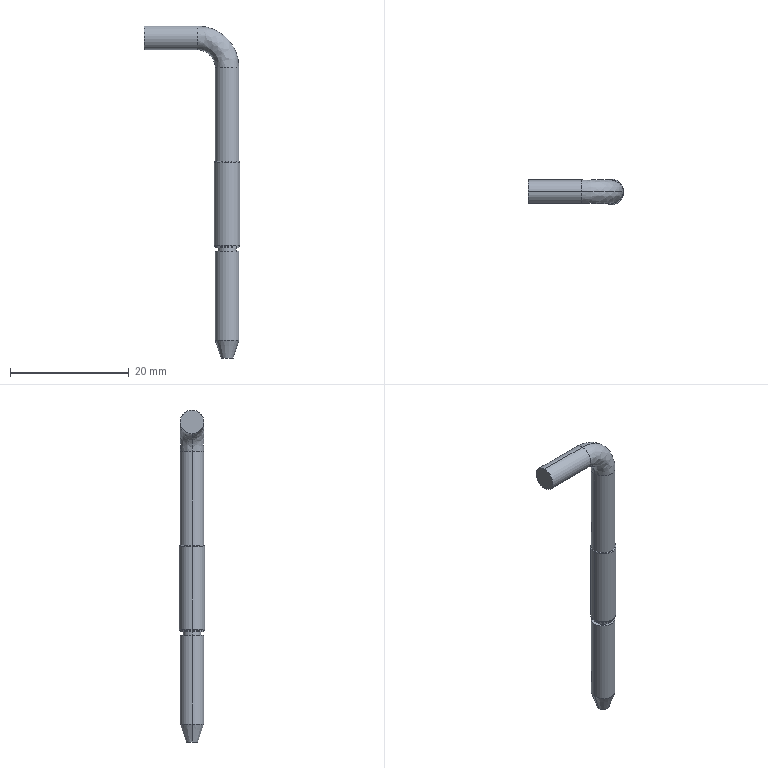Part | SolidWorks | features MirrorStock 1 | 1 solid | 24 faces | box 16.15 x 4.3 x 56 mm | volume 836.376 mm3 | cylinder 12 | spline 6 | plane 4 | cone 2 | commonest cylinder face diameters 4 x8 3 x2 4.3 x2
STEP:
#1=CARTESIAN_POINT('',(-2.,4.,7.15));
#2=VERTEX_POINT('',#1);
#3=CARTESIAN_POINT('',(2.,4.,7.15));
#4=VERTEX_POINT('',#3);
#5=CARTESIAN_POINT('',(0.,4.,7.15));
#6=DIRECTION('',(0.,0.,-1.));
#7=DIRECTION('',(-1.,0.,0.));
#8=AXIS2_PLACEMENT_3D('',#5,#6,#7);
#9=CIRCLE('',#8,2.);
#10=EDGE_CURVE('',#2,#4,#9,.T.);
#11=ORIENTED_EDGE('',*,*,#10,.T.);
#12=CARTESIAN_POINT('',(2.15,4.,7.));
#13=VERTEX_POINT('',#12);
#14=CARTESIAN_POINT('',(2.,4.,7.));
#15=DIRECTION('',(0.,1.,0.));
#16=DIRECTION('',(1.,0.,0.));
#17=AXIS2_PLACEMENT_3D('',#14,#15,#16);
#18=CIRCLE('',#17,0.15);
#19=EDGE_CURVE('',#4,#13,#18,.T.);
#20=ORIENTED_EDGE('',*,*,#19,.T.);
#21=CARTESIAN_POINT('',(-2.15,4.,7.));
#22=VERTEX_POINT('',#21);
#23=CARTESIAN_POINT('',(0.,4.,7.));
#24=DIRECTION('',(0.,0.,-1.));
#25=DIRECTION('',(-1.,0.,0.));
#26=AXIS2_PLACEMENT_3D('',#23,#24,#25);
#27=CIRCLE('',#26,2.15);
#28=EDGE_CURVE('',#22,#13,#27,.T.);
#29=ORIENTED_EDGE('',*,*,#28,.F.);
#30=CARTESIAN_POINT('',(-2.,4.,7.));
#31=DIRECTION('',(0.,-1.,0.));
#32=DIRECTION('',(-1.,0.,0.));
#33=AXIS2_PLACEMENT_3D('',#30,#31,#32);
#34=CIRCLE('',#33,0.15);
#35=EDGE_CURVE('',#2,#22,#34,.T.);
#36=ORIENTED_EDGE('',*,*,#35,.F.);
#37=EDGE_LOOP('',(#11,#20,#29,#36));
#38=FACE_OUTER_BOUND('',#37,.T.);
#39=CARTESIAN_POINT('',(2.,4.,7.15));
#40=CARTESIAN_POINT('',(2.,8.,7.15));
#41=CARTESIAN_POINT('',(-2.,8.,7.15));
#42=CARTESIAN_POINT('',(-2.,4.,7.15));
#43=CARTESIAN_POINT('',(2.088,4.,7.15));
#44=CARTESIAN_POINT('',(2.088,8.176,7.15));
#45=CARTESIAN_POINT('',(-2.088,8.176,7.15));
#46=CARTESIAN_POINT('',(-2.088,4.,7.15));
#47=CARTESIAN_POINT('',(2.15,4.,7.088));
#48=CARTESIAN_POINT('',(2.15,8.3,7.088));
#49=CARTESIAN_POINT('',(-2.15,8.3,7.088));
#50=CARTESIAN_POINT('',(-2.15,4.,7.088));
#51=CARTESIAN_POINT('',(2.15,4.,7.));
#52=CARTESIAN_POINT('',(2.15,8.3,7.));
#53=CARTESIAN_POINT('',(-2.15,8.3,7.));
#54=CARTESIAN_POINT('',(-2.15,4.,7.));
#55=(BOUNDED_SURFACE()B_SPLINE_SURFACE(3,3,((#39,#40,#41,#42),(#43,#44,#45,#46),(#47,#48,#49,#50),(#51,#52,#53,#54)),.UNSPECIFIED.,.F.,.F.,.T.)B_SPLINE_SURFACE_WITH_KNOTS((4,4),(4,4),(0.,1.),(0.,1.),.UNSPECIFIED.)GEOMETRIC_REPRESENTATION_ITEM()RATIONAL_B_SPLINE_SURFACE(((1.,0.3333,0.3333,1.),(0.8047,0.2682,0.2682,0.8047),(0.8047,0.2682,0.2682,0.8047),(1.,0.3333,0.3333,1.)))REPRESENTATION_ITEM('')SURFACE());
#56=ADVANCED_FACE('',(#38),#55,.T.);
#57=CARTESIAN_POINT('',(-2.15,4.,-7.));
#58=VERTEX_POINT('',#57);
#59=CARTESIAN_POINT('',(2.15,4.,-7.));
#60=VERTEX_POINT('',#59);
#61=CARTESIAN_POINT('',(0.,4.,-7.));
#62=DIRECTION('',(0.,0.,-1.));
#63=DIRECTION('',(-1.,0.,0.));
#64=AXIS2_PLACEMENT_3D('',#61,#62,#63);
#65=CIRCLE('',#64,2.15);
#66=EDGE_CURVE('',#58,#60,#65,.T.);
#67=ORIENTED_EDGE('',*,*,#66,.T.);
#68=CARTESIAN_POINT('',(2.,4.,-7.15));
#69=VERTEX_POINT('',#68);
#70=CARTESIAN_POINT('',(2.,4.,-7.));
#71=DIRECTION('',(0.,1.,0.));
#72=DIRECTION('',(1.,0.,0.));
#73=AXIS2_PLACEMENT_3D('',#70,#71,#72);
#74=CIRCLE('',#73,0.15);
#75=EDGE_CURVE('',#60,#69,#74,.T.);
#76=ORIENTED_EDGE('',*,*,#75,.T.);
#77=CARTESIAN_POINT('',(-2.,4.,-7.15));
#78=VERTEX_POINT('',#77);
#79=CARTESIAN_POINT('',(0.,4.,-7.15));
#80=DIRECTION('',(0.,0.,-1.));
#81=DIRECTION('',(-1.,0.,0.));
#82=AXIS2_PLACEMENT_3D('',#79,#80,#81);
#83=CIRCLE('',#82,2.);
#84=EDGE_CURVE('',#78,#69,#83,.T.);
#85=ORIENTED_EDGE('',*,*,#84,.F.);
#86=CARTESIAN_POINT('',(-2.,4.,-7.));
#87=DIRECTION('',(0.,-1.,0.));
#88=DIRECTION('',(-1.,0.,0.));
#89=AXIS2_PLACEMENT_3D('',#86,#87,#88);
#90=CIRCLE('',#89,0.15);
#91=EDGE_CURVE('',#58,#78,#90,.T.);
#92=ORIENTED_EDGE('',*,*,#91,.F.);
#93=EDGE_LOOP('',(#67,#76,#85,#92));
#94=FACE_OUTER_BOUND('',#93,.T.);
#95=CARTESIAN_POINT('',(2.15,4.,-7.));
#96=CARTESIAN_POINT('',(2.15,8.3,-7.));
#97=CARTESIAN_POINT('',(-2.15,8.3,-7.));
#98=CARTESIAN_POINT('',(-2.15,4.,-7.));
#99=CARTESIAN_POINT('',(2.15,4.,-7.088));
#100=CARTESIAN_POINT('',(2.15,8.3,-7.088));
#101=CARTESIAN_POINT('',(-2.15,8.3,-7.088));
#102=CARTESIAN_POINT('',(-2.15,4.,-7.088));
#103=CARTESIAN_POINT('',(2.088,4.,-7.15));
#104=CARTESIAN_POINT('',(2.088,8.176,-7.15));
#105=CARTESIAN_POINT('',(-2.088,8.176,-7.15));
#106=CARTESIAN_POINT('',(-2.088,4.,-7.15));
#107=CARTESIAN_POINT('',(2.,4.,-7.15));
#108=CARTESIAN_POINT('',(2.,8.,-7.15));
#109=CARTESIAN_POINT('',(-2.,8.,-7.15));
#110=CARTESIAN_POINT('',(-2.,4.,-7.15));
#111=(BOUNDED_SURFACE()B_SPLINE_SURFACE(3,3,((#95,#96,#97,#98),(#99,#100,#101,#102),(#103,#104,#105,#106),(#107,#108,#109,#110)),.UNSPECIFIED.,.F.,.F.,.T.)B_SPLINE_SURFACE_WITH_KNOTS((4,4),(4,4),(0.,1.),(0.,1.),.UNSPECIFIED.)GEOMETRIC_REPRESENTATION_ITEM()RATIONAL_B_SPLINE_SURFACE(((1.,0.3333,0.3333,1.),(0.8047,0.2682,0.2682,0.8047),(0.8047,0.2682,0.2682,0.8047),(1.,0.3333,0.3333,1.)))REPRESENTATION_ITEM('')SURFACE());
#112=ADVANCED_FACE('',(#94),#111,.T.);
#113=CARTESIAN_POINT('',(0.,4.,7.15));
#114=DIRECTION('',(0.,0.,-1.));
#115=DIRECTION('',(-1.,0.,0.));
#116=AXIS2_PLACEMENT_3D('',#113,#114,#115);
#117=CIRCLE('',#116,2.);
#118=EDGE_CURVE('',#4,#2,#117,.T.);
#119=ORIENTED_EDGE('',*,*,#118,.F.);
#120=CARTESIAN_POINT('',(2.,4.,23.));
#121=VERTEX_POINT('',#120);
#122=CARTESIAN_POINT('',(2.,4.,23.));
#123=DIRECTION('',(0.,0.,1.));
#124=VECTOR('',#123,1000.);
#125=LINE('',#122,#124);
#126=EDGE_CURVE('',#4,#121,#125,.T.);
#127=ORIENTED_EDGE('',*,*,#126,.T.);
#128=CARTESIAN_POINT('',(-2.,4.,23.));
#129=VERTEX_POINT('',#128);
#130=CARTESIAN_POINT('',(0.,4.,23.));
#131=DIRECTION('',(0.,0.,1.));
#132=DIRECTION('',(-1.,0.,0.));
#133=AXIS2_PLACEMENT_3D('',#130,#131,#132);
#134=CIRCLE('',#133,2.);
#135=EDGE_CURVE('',#129,#121,#134,.T.);
#136=ORIENTED_EDGE('',*,*,#135,.F.);
#137=CARTESIAN_POINT('',(-2.,4.,23.));
#138=DIRECTION('',(0.,0.,1.));
#139=VECTOR('',#138,1000.);
#140=LINE('',#137,#139);
#141=EDGE_CURVE('',#2,#129,#140,.T.);
#142=ORIENTED_EDGE('',*,*,#141,.F.);
#143=EDGE_LOOP('',(#119,#127,#136,#142));
#144=FACE_OUTER_BOUND('',#143,.T.);
#145=CARTESIAN_POINT('',(0.,4.,23.));
#146=DIRECTION('',(0.,0.,1.));
#147=DIRECTION('',(-1.,0.,0.));
#148=AXIS2_PLACEMENT_3D('',#145,#146,#147);
#149=CYLINDRICAL_SURFACE('',#148,2.);
#150=ADVANCED_FACE('',(#144),#149,.T.);
#151=CARTESIAN_POINT('',(-5.,4.,26.));
#152=VERTEX_POINT('',#151);
#153=CARTESIAN_POINT('',(-5.,4.,30.));
#154=VERTEX_POINT('',#153);
#155=CARTESIAN_POINT('',(-5.,4.,28.));
#156=DIRECTION('',(-1.,0.,0.));
#157=DIRECTION('',(0.,0.,1.));
#158=AXIS2_PLACEMENT_3D('',#155,#156,#157);
#159=CIRCLE('',#158,2.);
#160=EDGE_CURVE('',#152,#154,#159,.T.);
#161=ORIENTED_EDGE('',*,*,#160,.F.);
#162=CARTESIAN_POINT('',(-5.,4.,23.));
#163=DIRECTION('',(0.,1.,0.));
#164=DIRECTION('',(0.,0.,-1.));
#165=AXIS2_PLACEMENT_3D('',#162,#163,#164);
#166=CIRCLE('',#165,3.);
#167=EDGE_CURVE('',#152,#129,#166,.T.);
#168=ORIENTED_EDGE('',*,*,#167,.T.);
#169=ORIENTED_EDGE('',*,*,#135,.T.);
#170=CARTESIAN_POINT('',(-5.,4.,23.));
#171=DIRECTION('',(0.,1.,0.));
#172=DIRECTION('',(0.,0.,-1.));
#173=AXIS2_PLACEMENT_3D('',#170,#171,#172);
#174=CIRCLE('',#173,7.);
#175=EDGE_CURVE('',#154,#121,#174,.T.);
#176=ORIENTED_EDGE('',*,*,#175,.F.);
#177=EDGE_LOOP('',(#161,#168,#169,#176));
#178=FACE_OUTER_BOUND('',#177,.T.);
#179=CARTESIAN_POINT('',(-5.,4.,30.));
#180=CARTESIAN_POINT('',(-0.8995,4.,30.));
#181=CARTESIAN_POINT('',(2.,4.,27.101));
#182=CARTESIAN_POINT('',(2.,4.,23.));
#183=CARTESIAN_POINT('',(-5.,0.,30.));
#184=CARTESIAN_POINT('',(-0.8995,0.,30.));
#185=CARTESIAN_POINT('',(2.,0.,27.101));
#186=CARTESIAN_POINT('',(2.,0.,23.));
#187=CARTESIAN_POINT('',(-5.,0.,26.));
#188=CARTESIAN_POINT('',(-3.243,0.,26.));
#189=CARTESIAN_POINT('',(-2.,0.,24.757));
#190=CARTESIAN_POINT('',(-2.,0.,23.));
#191=CARTESIAN_POINT('',(-5.,4.,26.));
#192=CARTESIAN_POINT('',(-3.243,4.,26.));
#193=CARTESIAN_POINT('',(-2.,4.,24.757));
#194=CARTESIAN_POINT('',(-2.,4.,23.));
#195=(BOUNDED_SURFACE()B_SPLINE_SURFACE(3,3,((#179,#180,#181,#182),(#183,#184,#185,#186),(#187,#188,#189,#190),(#191,#192,#193,#194)),.UNSPECIFIED.,.F.,.F.,.T.)B_SPLINE_SURFACE_WITH_KNOTS((4,4),(4,4),(0.,1.),(0.,1.),.UNSPECIFIED.)GEOMETRIC_REPRESENTATION_ITEM()RATIONAL_B_SPLINE_SURFACE(((1.,0.8047,0.8047,1.),(0.3333,0.2682,0.2682,0.3333),(0.3333,0.2682,0.2682,0.3333),(1.,0.8047,0.8047,1.)))REPRESENTATION_ITEM('')SURFACE());
#196=ADVANCED_FACE('',(#178),#195,.T.);
#197=CARTESIAN_POINT('',(0.,4.,-7.));
#198=DIRECTION('',(0.,0.,-1.));
#199=DIRECTION('',(-1.,0.,0.));
#200=AXIS2_PLACEMENT_3D('',#197,#198,#199);
#201=CIRCLE('',#200,2.15);
#202=EDGE_CURVE('',#60,#58,#201,.T.);
#203=ORIENTED_EDGE('',*,*,#202,.F.);
#204=CARTESIAN_POINT('',(2.15,4.,-7.));
#205=DIRECTION('',(0.,0.,1.));
#206=VECTOR('',#205,1000.);
#207=LINE('',#204,#206);
#208=EDGE_CURVE('',#60,#13,#207,.T.);
#209=ORIENTED_EDGE('',*,*,#208,.T.);
#210=CARTESIAN_POINT('',(0.,4.,7.));
#211=DIRECTION('',(0.,0.,-1.));
#212=DIRECTION('',(-1.,0.,0.));
#213=AXIS2_PLACEMENT_3D('',#210,#211,#212);
#214=CIRCLE('',#213,2.15);
#215=EDGE_CURVE('',#13,#22,#214,.T.);
#216=ORIENTED_EDGE('',*,*,#215,.T.);
#217=CARTESIAN_POINT('',(-2.15,4.,-7.));
#218=DIRECTION('',(0.,0.,1.));
#219=VECTOR('',#218,1000.);
#220=LINE('',#217,#219);
#221=EDGE_CURVE('',#58,#22,#220,.T.);
#222=ORIENTED_EDGE('',*,*,#221,.F.);
#223=EDGE_LOOP('',(#203,#209,#216,#222));
#224=FACE_OUTER_BOUND('',#223,.T.);
#225=CARTESIAN_POINT('',(0.,4.,-7.));
#226=DIRECTION('',(0.,0.,1.));
#227=DIRECTION('',(-1.,0.,0.));
#228=AXIS2_PLACEMENT_3D('',#225,#226,#227);
#229=CYLINDRICAL_SURFACE('',#228,2.15);
#230=ADVANCED_FACE('',(#224),#229,.T.);
#231=CARTESIAN_POINT('',(-14.,4.,26.));
#232=VERTEX_POINT('',#231);
#233=CARTESIAN_POINT('',(-14.,4.,30.));
#234=VERTEX_POINT('',#233);
#235=CARTESIAN_POINT('',(-14.,4.,28.));
#236=DIRECTION('',(-1.,0.,0.));
#237=DIRECTION('',(0.,0.,1.));
#238=AXIS2_PLACEMENT_3D('',#235,#236,#237);
#239=CIRCLE('',#238,2.);
#240=EDGE_CURVE('',#232,#234,#239,.T.);
#241=ORIENTED_EDGE('',*,*,#240,.F.);
#242=CARTESIAN_POINT('',(-14.,4.,26.));
#243=DIRECTION('',(1.,0.,0.));
#244=VECTOR('',#243,1000.);
#245=LINE('',#242,#244);
#246=EDGE_CURVE('',#232,#152,#245,.T.);
#247=ORIENTED_EDGE('',*,*,#246,.T.);
#248=ORIENTED_EDGE('',*,*,#160,.T.);
#249=CARTESIAN_POINT('',(-14.,4.,30.));
#250=DIRECTION('',(1.,0.,0.));
#251=VECTOR('',#250,1000.);
#252=LINE('',#249,#251);
#253=EDGE_CURVE('',#234,#154,#252,.T.);
#254=ORIENTED_EDGE('',*,*,#253,.F.);
#255=EDGE_LOOP('',(#241,#247,#248,#254));
#256=FACE_OUTER_BOUND('',#255,.T.);
#257=CARTESIAN_POINT('',(-14.,4.,28.));
#258=DIRECTION('',(1.,0.,0.));
#259=DIRECTION('',(0.,0.,1.));
#260=AXIS2_PLACEMENT_3D('',#257,#258,#259);
#261=CYLINDRICAL_SURFACE('',#260,2.);
#262=ADVANCED_FACE('',(#256),#261,.T.);
#263=CARTESIAN_POINT('',(2.,4.,-7.4));
#264=VERTEX_POINT('',#263);
#265=CARTESIAN_POINT('',(-2.,4.,-7.4));
#266=VERTEX_POINT('',#265);
#267=CARTESIAN_POINT('',(0.,4.,-7.4));
#268=DIRECTION('',(0.,0.,-1.));
#269=DIRECTION('',(-1.,0.,0.));
#270=AXIS2_PLACEMENT_3D('',#267,#268,#269);
#271=CIRCLE('',#270,2.);
#272=EDGE_CURVE('',#264,#266,#271,.T.);
#273=ORIENTED_EDGE('',*,*,#272,.F.);
#274=CARTESIAN_POINT('',(2.,4.,23.));
#275=DIRECTION('',(0.,0.,1.));
#276=VECTOR('',#275,1000.);
#277=LINE('',#274,#276);
#278=EDGE_CURVE('',#264,#69,#277,.T.);
#279=ORIENTED_EDGE('',*,*,#278,.T.);
#280=CARTESIAN_POINT('',(0.,4.,-7.15));
#281=DIRECTION('',(0.,0.,-1.));
#282=DIRECTION('',(-1.,0.,0.));
#283=AXIS2_PLACEMENT_3D('',#280,#281,#282);
#284=CIRCLE('',#283,2.);
#285=EDGE_CURVE('',#69,#78,#284,.T.);
#286=ORIENTED_EDGE('',*,*,#285,.T.);
#287=CARTESIAN_POINT('',(-2.,4.,23.));
#288=DIRECTION('',(0.,0.,1.));
#289=VECTOR('',#288,1000.);
#290=LINE('',#287,#289);
#291=EDGE_CURVE('',#266,#78,#290,.T.);
#292=ORIENTED_EDGE('',*,*,#291,.F.);
#293=EDGE_LOOP('',(#273,#279,#286,#292));
#294=FACE_OUTER_BOUND('',#293,.T.);
#295=CARTESIAN_POINT('',(0.,4.,23.));
#296=DIRECTION('',(0.,0.,1.));
#297=DIRECTION('',(-1.,0.,0.));
#298=AXIS2_PLACEMENT_3D('',#295,#296,#297);
#299=CYLINDRICAL_SURFACE('',#298,2.);
#300=ADVANCED_FACE('',(#294),#299,.T.);
#301=CARTESIAN_POINT('',(-1.5,4.,-7.4));
#302=VERTEX_POINT('',#301);
#303=CARTESIAN_POINT('',(1.5,4.,-7.4));
#304=VERTEX_POINT('',#303);
#305=CARTESIAN_POINT('',(0.,4.,-7.4));
#306=DIRECTION('',(0.,0.,1.));
#307=DIRECTION('',(1.,0.,0.));
#308=AXIS2_PLACEMENT_3D('',#305,#306,#307);
#309=CIRCLE('',#308,1.5);
#310=EDGE_CURVE('',#302,#304,#309,.T.);
#311=ORIENTED_EDGE('',*,*,#310,.F.);
#312=CARTESIAN_POINT('',(-1.5,4.,-8.));
#313=VERTEX_POINT('',#312);
#314=CARTESIAN_POINT('',(-1.5,4.,-50.));
#315=DIRECTION('',(0.,0.,-1.));
#316=VECTOR('',#315,1000.);
#317=LINE('',#314,#316);
#318=EDGE_CURVE('',#302,#313,#317,.T.);
#319=ORIENTED_EDGE('',*,*,#318,.T.);
#320=CARTESIAN_POINT('',(1.5,4.,-8.));
#321=VERTEX_POINT('',#320);
#322=CARTESIAN_POINT('',(0.,4.,-8.));
#323=DIRECTION('',(0.,0.,-1.));
#324=DIRECTION('',(1.,0.,0.));
#325=AXIS2_PLACEMENT_3D('',#322,#323,#324);
#326=CIRCLE('',#325,1.5);
#327=EDGE_CURVE('',#321,#313,#326,.T.);
#328=ORIENTED_EDGE('',*,*,#327,.F.);
#329=CARTESIAN_POINT('',(1.5,4.,-50.));
#330=DIRECTION('',(0.,0.,-1.));
#331=VECTOR('',#330,1000.);
#332=LINE('',#329,#331);
#333=EDGE_CURVE('',#304,#321,#332,.T.);
#334=ORIENTED_EDGE('',*,*,#333,.F.);
#335=EDGE_LOOP('',(#311,#319,#328,#334));
#336=FACE_OUTER_BOUND('',#335,.T.);
#337=CARTESIAN_POINT('',(0.,4.,-50.));
#338=DIRECTION('',(0.,0.,-1.));
#339=DIRECTION('',(1.,0.,0.));
#340=AXIS2_PLACEMENT_3D('',#337,#338,#339);
#341=CYLINDRICAL_SURFACE('',#340,1.5);
#342=ADVANCED_FACE('',(#336),#341,.T.);
#343=CARTESIAN_POINT('',(2.,4.,-23.));
#344=VERTEX_POINT('',#343);
#345=CARTESIAN_POINT('',(-2.,4.,-23.));
#346=VERTEX_POINT('',#345);
#347=CARTESIAN_POINT('',(0.,4.,-23.));
#348=DIRECTION('',(0.,0.,-1.));
#349=DIRECTION('',(-1.,0.,0.));
#350=AXIS2_PLACEMENT_3D('',#347,#348,#349);
#351=CIRCLE('',#350,2.);
#352=EDGE_CURVE('',#344,#346,#351,.T.);
#353=ORIENTED_EDGE('',*,*,#352,.F.);
#354=CARTESIAN_POINT('',(2.,4.,-8.));
#355=VERTEX_POINT('',#354);
#356=CARTESIAN_POINT('',(2.,4.,23.));
#357=DIRECTION('',(0.,0.,1.));
#358=VECTOR('',#357,1000.);
#359=LINE('',#356,#358);
#360=EDGE_CURVE('',#344,#355,#359,.T.);
#361=ORIENTED_EDGE('',*,*,#360,.T.);
#362=CARTESIAN_POINT('',(-2.,4.,-8.));
#363=VERTEX_POINT('',#362);
#364=CARTESIAN_POINT('',(0.,4.,-8.));
#365=DIRECTION('',(0.,0.,1.));
#366=DIRECTION('',(-1.,0.,0.));
#367=AXIS2_PLACEMENT_3D('',#364,#365,#366);
#368=CIRCLE('',#367,2.);
#369=EDGE_CURVE('',#363,#355,#368,.T.);
#370=ORIENTED_EDGE('',*,*,#369,.F.);
#371=CARTESIAN_POINT('',(-2.,4.,23.));
#372=DIRECTION('',(0.,0.,1.));
#373=VECTOR('',#372,1000.);
#374=LINE('',#371,#373);
#375=EDGE_CURVE('',#346,#363,#374,.T.);
#376=ORIENTED_EDGE('',*,*,#375,.F.);
#377=EDGE_LOOP('',(#353,#361,#370,#376));
#378=FACE_OUTER_BOUND('',#377,.T.);
#379=CARTESIAN_POINT('',(0.,4.,23.));
#380=DIRECTION('',(0.,0.,1.));
#381=DIRECTION('',(-1.,0.,0.));
#382=AXIS2_PLACEMENT_3D('',#379,#380,#381);
#383=CYLINDRICAL_SURFACE('',#382,2.);
#384=ADVANCED_FACE('',(#378),#383,.T.);
#385=CARTESIAN_POINT('',(1.,4.,-26.));
#386=VERTEX_POINT('',#385);
#387=CARTESIAN_POINT('',(-1.,4.,-26.));
#388=VERTEX_POINT('',#387);
#389=CARTESIAN_POINT('',(0.,4.,-26.));
#390=DIRECTION('',(0.,0.,-1.));
#391=DIRECTION('',(-1.,0.,0.));
#392=AXIS2_PLACEMENT_3D('',#389,#390,#391);
#393=CIRCLE('',#392,1.);
#394=EDGE_CURVE('',#386,#388,#393,.T.);
#395=ORIENTED_EDGE('',*,*,#394,.F.);
#396=CARTESIAN_POINT('',(2.,4.,-23.));
#397=DIRECTION('',(0.3162,0.,0.9487));
#398=VECTOR('',#397,1000.);
#399=LINE('',#396,#398);
#400=EDGE_CURVE('',#386,#344,#399,.T.);
#401=ORIENTED_EDGE('',*,*,#400,.T.);
#402=ORIENTED_EDGE('',*,*,#352,.T.);
#403=CARTESIAN_POINT('',(-2.,4.,-23.));
#404=DIRECTION('',(-0.3162,0.,0.9487));
#405=VECTOR('',#404,1000.);
#406=LINE('',#403,#405);
#407=EDGE_CURVE('',#388,#346,#406,.T.);
#408=ORIENTED_EDGE('',*,*,#407,.F.);
#409=EDGE_LOOP('',(#395,#401,#402,#408));
#410=FACE_OUTER_BOUND('',#409,.T.);
#411=CARTESIAN_POINT('',(0.,4.,-23.));
#412=DIRECTION('',(0.,0.,1.));
#413=DIRECTION('',(-1.,0.,0.));
#414=AXIS2_PLACEMENT_3D('',#411,#412,#413);
#415=CONICAL_SURFACE('',#414,2.,0.3218);
#416=ADVANCED_FACE('',(#410),#415,.T.);
#417=CARTESIAN_POINT('',(0.,4.,-26.));
#418=DIRECTION('',(0.,0.,-1.));
#419=DIRECTION('',(-1.,0.,0.));
#420=AXIS2_PLACEMENT_3D('',#417,#418,#419);
#421=CIRCLE('',#420,1.);
#422=EDGE_CURVE('',#388,#386,#421,.T.);
#423=ORIENTED_EDGE('',*,*,#422,.T.);
#424=ORIENTED_EDGE('',*,*,#394,.T.);
#425=EDGE_LOOP('',(#423,#424));
#426=FACE_OUTER_BOUND('',#425,.T.);
#427=CARTESIAN_POINT('',(0.,4.,-26.));
#428=DIRECTION('',(0.,0.,1.));
#429=DIRECTION('',(-1.,0.,0.));
#430=AXIS2_PLACEMENT_3D('',#427,#428,#429);
#431=PLANE('',#430);
#432=ADVANCED_FACE('',(#426),#431,.F.);
#433=ORIENTED_EDGE('',*,*,#400,.F.);
#434=ORIENTED_EDGE('',*,*,#422,.F.);
#435=ORIENTED_EDGE('',*,*,#407,.T.);
#436=CARTESIAN_POINT('',(0.,4.,-23.));
#437=DIRECTION('',(0.,0.,-1.));
#438=DIRECTION('',(-1.,0.,0.));
#439=AXIS2_PLACEMENT_3D('',#436,#437,#438);
#440=CIRCLE('',#439,2.);
#441=EDGE_CURVE('',#346,#344,#440,.T.);
#442=ORIENTED_EDGE('',*,*,#441,.T.);
#443=EDGE_LOOP('',(#433,#434,#435,#442));
#444=FACE_OUTER_BOUND('',#443,.T.);
#445=CARTESIAN_POINT('',(0.,4.,-23.));
#446=DIRECTION('',(0.,0.,1.));
#447=DIRECTION('',(-1.,0.,0.));
#448=AXIS2_PLACEMENT_3D('',#445,#446,#447);
#449=CONICAL_SURFACE('',#448,2.,0.3218);
#450=ADVANCED_FACE('',(#444),#449,.T.);
#451=ORIENTED_EDGE('',*,*,#360,.F.);
#452=ORIENTED_EDGE('',*,*,#441,.F.);
#453=ORIENTED_EDGE('',*,*,#375,.T.);
#454=CARTESIAN_POINT('',(0.,4.,-8.));
#455=DIRECTION('',(0.,0.,1.));
#456=DIRECTION('',(-1.,0.,0.));
#457=AXIS2_PLACEMENT_3D('',#454,#455,#456);
#458=CIRCLE('',#457,2.);
#459=EDGE_CURVE('',#355,#363,#458,.T.);
#460=ORIENTED_EDGE('',*,*,#459,.F.);
#461=EDGE_LOOP('',(#451,#452,#453,#460));
#462=FACE_OUTER_BOUND('',#461,.T.);
#463=CARTESIAN_POINT('',(0.,4.,23.));
#464=DIRECTION('',(0.,0.,1.));
#465=DIRECTION('',(-1.,0.,0.));
#466=AXIS2_PLACEMENT_3D('',#463,#464,#465);
#467=CYLINDRICAL_SURFACE('',#466,2.);
#468=ADVANCED_FACE('',(#462),#467,.T.);
#469=ORIENTED_EDGE('',*,*,#327,.T.);
#470=CARTESIAN_POINT('',(0.,4.,-8.));
#471=DIRECTION('',(0.,0.,-1.));
#472=DIRECTION('',(1.,0.,0.));
#473=AXIS2_PLACEMENT_3D('',#470,#471,#472);
#474=CIRCLE('',#473,1.5);
#475=EDGE_CURVE('',#313,#321,#474,.T.);
#476=ORIENTED_EDGE('',*,*,#475,.T.);
#477=EDGE_LOOP('',(#469,#476));
#478=FACE_BOUND('',#477,.T.);
#479=ORIENTED_EDGE('',*,*,#369,.T.);
#480=ORIENTED_EDGE('',*,*,#459,.T.);
#481=EDGE_LOOP('',(#479,#480));
#482=FACE_OUTER_BOUND('',#481,.T.);
#483=CARTESIAN_POINT('',(1.5,4.,-8.));
#484=DIRECTION('',(0.,0.,-1.));
#485=DIRECTION('',(1.,0.,0.));
#486=AXIS2_PLACEMENT_3D('',#483,#484,#485);
#487=PLANE('',#486);
#488=ADVANCED_FACE('',(#478,#482),#487,.F.);
#489=ORIENTED_EDGE('',*,*,#318,.F.);
#490=CARTESIAN_POINT('',(0.,4.,-7.4));
#491=DIRECTION('',(0.,0.,1.));
#492=DIRECTION('',(1.,0.,0.));
#493=AXIS2_PLACEMENT_3D('',#490,#491,#492);
#494=CIRCLE('',#493,1.5);
#495=EDGE_CURVE('',#304,#302,#494,.T.);
#496=ORIENTED_EDGE('',*,*,#495,.F.);
#497=ORIENTED_EDGE('',*,*,#333,.T.);
#498=ORIENTED_EDGE('',*,*,#475,.F.);
#499=EDGE_LOOP('',(#489,#496,#497,#498));
#500=FACE_OUTER_BOUND('',#499,.T.);
#501=CARTESIAN_POINT('',(0.,4.,-50.));
#502=DIRECTION('',(0.,0.,-1.));
#503=DIRECTION('',(1.,0.,0.));
#504=AXIS2_PLACEMENT_3D('',#501,#502,#503);
#505=CYLINDRICAL_SURFACE('',#504,1.5);
#506=ADVANCED_FACE('',(#500),#505,.T.);
#507=CARTESIAN_POINT('',(0.,4.,-7.4));
#508=DIRECTION('',(0.,0.,-1.));
#509=DIRECTION('',(-1.,0.,0.));
#510=AXIS2_PLACEMENT_3D('',#507,#508,#509);
#511=CIRCLE('',#510,2.);
#512=EDGE_CURVE('',#266,#264,#511,.T.);
#513=ORIENTED_EDGE('',*,*,#512,.T.);
#514=ORIENTED_EDGE('',*,*,#272,.T.);
#515=EDGE_LOOP('',(#513,#514));
#516=FACE_OUTER_BOUND('',#515,.T.);
#517=ORIENTED_EDGE('',*,*,#495,.T.);
#518=ORIENTED_EDGE('',*,*,#310,.T.);
#519=EDGE_LOOP('',(#517,#518));
#520=FACE_BOUND('',#519,.T.);
#521=CARTESIAN_POINT('',(4.,4.,-7.4));
#522=DIRECTION('',(0.,0.,1.));
#523=DIRECTION('',(-1.,0.,0.));
#524=AXIS2_PLACEMENT_3D('',#521,#522,#523);
#525=PLANE('',#524);
#526=ADVANCED_FACE('',(#516,#520),#525,.F.);
#527=ORIENTED_EDGE('',*,*,#278,.F.);
#528=ORIENTED_EDGE('',*,*,#512,.F.);
#529=ORIENTED_EDGE('',*,*,#291,.T.);
#530=ORIENTED_EDGE('',*,*,#84,.T.);
#531=EDGE_LOOP('',(#527,#528,#529,#530));
#532=FACE_OUTER_BOUND('',#531,.T.);
#533=CARTESIAN_POINT('',(0.,4.,23.));
#534=DIRECTION('',(0.,0.,1.));
#535=DIRECTION('',(-1.,0.,0.));
#536=AXIS2_PLACEMENT_3D('',#533,#534,#535);
#537=CYLINDRICAL_SURFACE('',#536,2.);
#538=ADVANCED_FACE('',(#532),#537,.T.);
#539=CARTESIAN_POINT('',(-14.,4.,28.));
#540=DIRECTION('',(-1.,0.,0.));
#541=DIRECTION('',(0.,0.,1.));
#542=AXIS2_PLACEMENT_3D('',#539,#540,#541);
#543=CIRCLE('',#542,2.);
#544=EDGE_CURVE('',#234,#232,#543,.T.);
#545=ORIENTED_EDGE('',*,*,#544,.T.);
#546=ORIENTED_EDGE('',*,*,#240,.T.);
#547=EDGE_LOOP('',(#545,#546));
#548=FACE_OUTER_BOUND('',#547,.T.);
#549=CARTESIAN_POINT('',(-14.,4.,28.));
#550=DIRECTION('',(-1.,0.,0.));
#551=DIRECTION('',(0.,0.,-1.));
#552=AXIS2_PLACEMENT_3D('',#549,#550,#551);
#553=PLANE('',#552);
#554=ADVANCED_FACE('',(#548),#553,.T.);
#555=ORIENTED_EDGE('',*,*,#75,.F.);
#556=ORIENTED_EDGE('',*,*,#202,.T.);
#557=ORIENTED_EDGE('',*,*,#91,.T.);
#558=ORIENTED_EDGE('',*,*,#285,.F.);
#559=EDGE_LOOP('',(#555,#556,#557,#558));
#560=FACE_OUTER_BOUND('',#559,.T.);
#561=CARTESIAN_POINT('',(-2.15,4.,-7.));
#562=CARTESIAN_POINT('',(-2.15,-0.3,-7.));
#563=CARTESIAN_POINT('',(2.15,-0.3,-7.));
#564=CARTESIAN_POINT('',(2.15,4.,-7.));
#565=CARTESIAN_POINT('',(-2.15,4.,-7.088));
#566=CARTESIAN_POINT('',(-2.15,-0.3,-7.088));
#567=CARTESIAN_POINT('',(2.15,-0.3,-7.088));
#568=CARTESIAN_POINT('',(2.15,4.,-7.088));
#569=CARTESIAN_POINT('',(-2.088,4.,-7.15));
#570=CARTESIAN_POINT('',(-2.088,-0.1757,-7.15));
#571=CARTESIAN_POINT('',(2.088,-0.1757,-7.15));
#572=CARTESIAN_POINT('',(2.088,4.,-7.15));
#573=CARTESIAN_POINT('',(-2.,4.,-7.15));
#574=CARTESIAN_POINT('',(-2.,0.,-7.15));
#575=CARTESIAN_POINT('',(2.,0.,-7.15));
#576=CARTESIAN_POINT('',(2.,4.,-7.15));
#577=(BOUNDED_SURFACE()B_SPLINE_SURFACE(3,3,((#561,#562,#563,#564),(#565,#566,#567,#568),(#569,#570,#571,#572),(#573,#574,#575,#576)),.UNSPECIFIED.,.F.,.F.,.T.)B_SPLINE_SURFACE_WITH_KNOTS((4,4),(4,4),(0.,1.),(0.,1.),.UNSPECIFIED.)GEOMETRIC_REPRESENTATION_ITEM()RATIONAL_B_SPLINE_SURFACE(((1.,0.3333,0.3333,1.),(0.8047,0.2682,0.2682,0.8047),(0.8047,0.2682,0.2682,0.8047),(1.,0.3333,0.3333,1.)))REPRESENTATION_ITEM('')SURFACE());
#578=ADVANCED_FACE('',(#560),#577,.T.);
#579=ORIENTED_EDGE('',*,*,#246,.F.);
#580=ORIENTED_EDGE('',*,*,#544,.F.);
#581=ORIENTED_EDGE('',*,*,#253,.T.);
#582=CARTESIAN_POINT('',(-5.,4.,28.));
#583=DIRECTION('',(-1.,0.,0.));
#584=DIRECTION('',(0.,0.,1.));
#585=AXIS2_PLACEMENT_3D('',#582,#583,#584);
#586=CIRCLE('',#585,2.);
#587=EDGE_CURVE('',#154,#152,#586,.T.);
#588=ORIENTED_EDGE('',*,*,#587,.T.);
#589=EDGE_LOOP('',(#579,#580,#581,#588));
#590=FACE_OUTER_BOUND('',#589,.T.);
#591=CARTESIAN_POINT('',(-14.,4.,28.));
#592=DIRECTION('',(1.,0.,0.));
#593=DIRECTION('',(0.,0.,1.));
#594=AXIS2_PLACEMENT_3D('',#591,#592,#593);
#595=CYLINDRICAL_SURFACE('',#594,2.);
#596=ADVANCED_FACE('',(#590),#595,.T.);
#597=ORIENTED_EDGE('',*,*,#208,.F.);
#598=ORIENTED_EDGE('',*,*,#66,.F.);
#599=ORIENTED_EDGE('',*,*,#221,.T.);
#600=ORIENTED_EDGE('',*,*,#28,.T.);
#601=EDGE_LOOP('',(#597,#598,#599,#600));
#602=FACE_OUTER_BOUND('',#601,.T.);
#603=CARTESIAN_POINT('',(0.,4.,-7.));
#604=DIRECTION('',(0.,0.,1.));
#605=DIRECTION('',(-1.,0.,0.));
#606=AXIS2_PLACEMENT_3D('',#603,#604,#605);
#607=CYLINDRICAL_SURFACE('',#606,2.15);
#608=ADVANCED_FACE('',(#602),#607,.T.);
#609=ORIENTED_EDGE('',*,*,#167,.F.);
#610=ORIENTED_EDGE('',*,*,#587,.F.);
#611=ORIENTED_EDGE('',*,*,#175,.T.);
#612=CARTESIAN_POINT('',(0.,4.,23.));
#613=DIRECTION('',(0.,0.,1.));
#614=DIRECTION('',(-1.,0.,0.));
#615=AXIS2_PLACEMENT_3D('',#612,#613,#614);
#616=CIRCLE('',#615,2.);
#617=EDGE_CURVE('',#121,#129,#616,.T.);
#618=ORIENTED_EDGE('',*,*,#617,.T.);
#619=EDGE_LOOP('',(#609,#610,#611,#618));
#620=FACE_OUTER_BOUND('',#619,.T.);
#621=CARTESIAN_POINT('',(-5.,4.,26.));
#622=CARTESIAN_POINT('',(-3.243,4.,26.));
#623=CARTESIAN_POINT('',(-2.,4.,24.757));
#624=CARTESIAN_POINT('',(-2.,4.,23.));
#625=CARTESIAN_POINT('',(-5.,8.,26.));
#626=CARTESIAN_POINT('',(-3.243,8.,26.));
#627=CARTESIAN_POINT('',(-2.,8.,24.757));
#628=CARTESIAN_POINT('',(-2.,8.,23.));
#629=CARTESIAN_POINT('',(-5.,8.,30.));
#630=CARTESIAN_POINT('',(-0.8995,8.,30.));
#631=CARTESIAN_POINT('',(2.,8.,27.101));
#632=CARTESIAN_POINT('',(2.,8.,23.));
#633=CARTESIAN_POINT('',(-5.,4.,30.));
#634=CARTESIAN_POINT('',(-0.8995,4.,30.));
#635=CARTESIAN_POINT('',(2.,4.,27.101));
#636=CARTESIAN_POINT('',(2.,4.,23.));
#637=(BOUNDED_SURFACE()B_SPLINE_SURFACE(3,3,((#621,#622,#623,#624),(#625,#626,#627,#628),(#629,#630,#631,#632),(#633,#634,#635,#636)),.UNSPECIFIED.,.F.,.F.,.T.)B_SPLINE_SURFACE_WITH_KNOTS((4,4),(4,4),(0.,1.),(0.,1.),.UNSPECIFIED.)GEOMETRIC_REPRESENTATION_ITEM()RATIONAL_B_SPLINE_SURFACE(((1.,0.8047,0.8047,1.),(0.3333,0.2682,0.2682,0.3333),(0.3333,0.2682,0.2682,0.3333),(1.,0.8047,0.8047,1.)))REPRESENTATION_ITEM('')SURFACE());
#638=ADVANCED_FACE('',(#620),#637,.T.);
#639=ORIENTED_EDGE('',*,*,#19,.F.);
#640=ORIENTED_EDGE('',*,*,#118,.T.);
#641=ORIENTED_EDGE('',*,*,#35,.T.);
#642=ORIENTED_EDGE('',*,*,#215,.F.);
#643=EDGE_LOOP('',(#639,#640,#641,#642));
#644=FACE_OUTER_BOUND('',#643,.T.);
#645=CARTESIAN_POINT('',(-2.,4.,7.15));
#646=CARTESIAN_POINT('',(-2.,0.,7.15));
#647=CARTESIAN_POINT('',(2.,0.,7.15));
#648=CARTESIAN_POINT('',(2.,4.,7.15));
#649=CARTESIAN_POINT('',(-2.088,4.,7.15));
#650=CARTESIAN_POINT('',(-2.088,-0.1757,7.15));
#651=CARTESIAN_POINT('',(2.088,-0.1757,7.15));
#652=CARTESIAN_POINT('',(2.088,4.,7.15));
#653=CARTESIAN_POINT('',(-2.15,4.,7.088));
#654=CARTESIAN_POINT('',(-2.15,-0.3,7.088));
#655=CARTESIAN_POINT('',(2.15,-0.3,7.088));
#656=CARTESIAN_POINT('',(2.15,4.,7.088));
#657=CARTESIAN_POINT('',(-2.15,4.,7.));
#658=CARTESIAN_POINT('',(-2.15,-0.3,7.));
#659=CARTESIAN_POINT('',(2.15,-0.3,7.));
#660=CARTESIAN_POINT('',(2.15,4.,7.));
#661=(BOUNDED_SURFACE()B_SPLINE_SURFACE(3,3,((#645,#646,#647,#648),(#649,#650,#651,#652),(#653,#654,#655,#656),(#657,#658,#659,#660)),.UNSPECIFIED.,.F.,.F.,.T.)B_SPLINE_SURFACE_WITH_KNOTS((4,4),(4,4),(0.,1.),(0.,1.),.UNSPECIFIED.)GEOMETRIC_REPRESENTATION_ITEM()RATIONAL_B_SPLINE_SURFACE(((1.,0.3333,0.3333,1.),(0.8047,0.2682,0.2682,0.8047),(0.8047,0.2682,0.2682,0.8047),(1.,0.3333,0.3333,1.)))REPRESENTATION_ITEM('')SURFACE());
#662=ADVANCED_FACE('',(#644),#661,.T.);
#663=ORIENTED_EDGE('',*,*,#126,.F.);
#664=ORIENTED_EDGE('',*,*,#10,.F.);
#665=ORIENTED_EDGE('',*,*,#141,.T.);
#666=ORIENTED_EDGE('',*,*,#617,.F.);
#667=EDGE_LOOP('',(#663,#664,#665,#666));
#668=FACE_OUTER_BOUND('',#667,.T.);
#669=CARTESIAN_POINT('',(0.,4.,23.));
#670=DIRECTION('',(0.,0.,1.));
#671=DIRECTION('',(-1.,0.,0.));
#672=AXIS2_PLACEMENT_3D('',#669,#670,#671);
#673=CYLINDRICAL_SURFACE('',#672,2.);
#674=ADVANCED_FACE('',(#668),#673,.T.);
#675=CLOSED_SHELL('',(#56,#112,#150,#196,#230,#262,#300,#342,#384,#416,#432,#450,#468,#488,#506,#526,#538,#554,#578,#596,#608,#638,#662,#674));
#676=MANIFOLD_SOLID_BREP('',#675);
#677=CARTESIAN_POINT('',(0.,0.,0.));
#678=DIRECTION('',(0.,0.,1.));
#679=DIRECTION('',(1.,0.,0.));
#680=AXIS2_PLACEMENT_3D('',#677,#678,#679);
#681=(LENGTH_UNIT()NAMED_UNIT(*)SI_UNIT(.MILLI.,.METRE.));
#682=UNCERTAINTY_MEASURE_WITH_UNIT(LENGTH_MEASURE(0.00001),#681,'','');
#683=(NAMED_UNIT(*)PLANE_ANGLE_UNIT()SI_UNIT($,.RADIAN.));
#684=(NAMED_UNIT(*)SI_UNIT($,.STERADIAN.)SOLID_ANGLE_UNIT());
#685=(GEOMETRIC_REPRESENTATION_CONTEXT(3)GLOBAL_UNCERTAINTY_ASSIGNED_CONTEXT((#682))GLOBAL_UNIT_ASSIGNED_CONTEXT((#681,#683,#684))REPRESENTATION_CONTEXT('',''));
#686=ADVANCED_BREP_SHAPE_REPRESENTATION('',(#676,#680),#685);